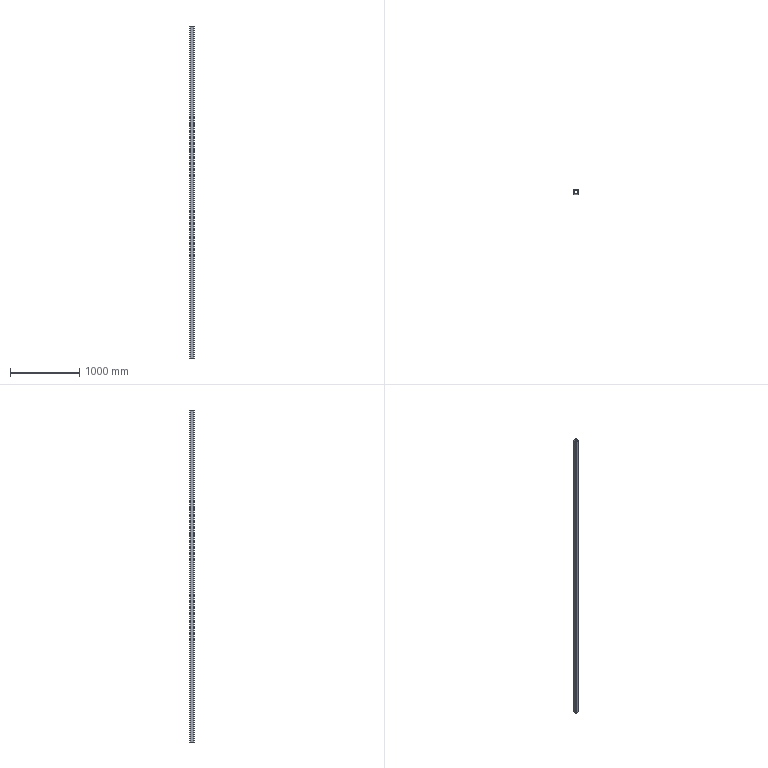Part | SolidWorks | features Extrusion 1 | 1 solid | 18 faces | box 64 x 64 x 4800 mm | volume 4410223 mm3 | plane 10 | cylinder 8 | commonest cylinder face diameters 8 x4 16 x4
STEP:
#1=CARTESIAN_POINT('',(-24.,32.,2400.));
#2=VERTEX_POINT('',#1);
#3=CARTESIAN_POINT('',(-32.,24.,2400.));
#4=VERTEX_POINT('',#3);
#5=CARTESIAN_POINT('',(-24.,24.,2400.));
#6=DIRECTION('',(0.,0.,1.));
#7=DIRECTION('',(1.,0.,0.));
#8=AXIS2_PLACEMENT_3D('',#5,#6,#7);
#9=CIRCLE('',#8,8.);
#10=EDGE_CURVE('',#2,#4,#9,.T.);
#11=ORIENTED_EDGE('',*,*,#10,.T.);
#12=CARTESIAN_POINT('',(-32.,-24.,2400.));
#13=VERTEX_POINT('',#12);
#14=CARTESIAN_POINT('',(-32.,24.,2400.));
#15=DIRECTION('',(0.,-1.,0.));
#16=VECTOR('',#15,1000.);
#17=LINE('',#14,#16);
#18=EDGE_CURVE('',#4,#13,#17,.T.);
#19=ORIENTED_EDGE('',*,*,#18,.T.);
#20=CARTESIAN_POINT('',(-24.,-32.,2400.));
#21=VERTEX_POINT('',#20);
#22=CARTESIAN_POINT('',(-24.,-24.,2400.));
#23=DIRECTION('',(0.,0.,1.));
#24=DIRECTION('',(-1.,0.,0.));
#25=AXIS2_PLACEMENT_3D('',#22,#23,#24);
#26=CIRCLE('',#25,8.);
#27=EDGE_CURVE('',#13,#21,#26,.T.);
#28=ORIENTED_EDGE('',*,*,#27,.T.);
#29=CARTESIAN_POINT('',(24.,-32.,2400.));
#30=VERTEX_POINT('',#29);
#31=CARTESIAN_POINT('',(24.,-32.,2400.));
#32=DIRECTION('',(1.,0.,0.));
#33=VECTOR('',#32,1000.);
#34=LINE('',#31,#33);
#35=EDGE_CURVE('',#21,#30,#34,.T.);
#36=ORIENTED_EDGE('',*,*,#35,.T.);
#37=CARTESIAN_POINT('',(32.,-24.,2400.));
#38=VERTEX_POINT('',#37);
#39=CARTESIAN_POINT('',(24.,-24.,2400.));
#40=DIRECTION('',(0.,0.,1.));
#41=DIRECTION('',(1.,0.,0.));
#42=AXIS2_PLACEMENT_3D('',#39,#40,#41);
#43=CIRCLE('',#42,8.);
#44=EDGE_CURVE('',#30,#38,#43,.T.);
#45=ORIENTED_EDGE('',*,*,#44,.T.);
#46=CARTESIAN_POINT('',(32.,24.,2400.));
#47=VERTEX_POINT('',#46);
#48=CARTESIAN_POINT('',(32.,-24.,2400.));
#49=DIRECTION('',(0.,1.,0.));
#50=VECTOR('',#49,1000.);
#51=LINE('',#48,#50);
#52=EDGE_CURVE('',#38,#47,#51,.T.);
#53=ORIENTED_EDGE('',*,*,#52,.T.);
#54=CARTESIAN_POINT('',(24.,32.,2400.));
#55=VERTEX_POINT('',#54);
#56=CARTESIAN_POINT('',(24.,24.,2400.));
#57=DIRECTION('',(0.,0.,1.));
#58=DIRECTION('',(-1.,0.,0.));
#59=AXIS2_PLACEMENT_3D('',#56,#57,#58);
#60=CIRCLE('',#59,8.);
#61=EDGE_CURVE('',#47,#55,#60,.T.);
#62=ORIENTED_EDGE('',*,*,#61,.T.);
#63=CARTESIAN_POINT('',(0.,32.,2400.));
#64=DIRECTION('',(-1.,0.,0.));
#65=VECTOR('',#64,1000.);
#66=LINE('',#63,#65);
#67=EDGE_CURVE('',#55,#2,#66,.T.);
#68=ORIENTED_EDGE('',*,*,#67,.T.);
#69=EDGE_LOOP('',(#11,#19,#28,#36,#45,#53,#62,#68));
#70=FACE_OUTER_BOUND('',#69,.T.);
#71=CARTESIAN_POINT('',(-28.,24.,2400.));
#72=VERTEX_POINT('',#71);
#73=CARTESIAN_POINT('',(-28.,-24.,2400.));
#74=VERTEX_POINT('',#73);
#75=CARTESIAN_POINT('',(-28.,24.,2400.));
#76=DIRECTION('',(0.,-1.,0.));
#77=VECTOR('',#76,1000.);
#78=LINE('',#75,#77);
#79=EDGE_CURVE('',#72,#74,#78,.T.);
#80=ORIENTED_EDGE('',*,*,#79,.F.);
#81=CARTESIAN_POINT('',(-24.,28.,2400.));
#82=VERTEX_POINT('',#81);
#83=CARTESIAN_POINT('',(-24.,24.,2400.));
#84=DIRECTION('',(0.,0.,1.));
#85=DIRECTION('',(1.,0.,0.));
#86=AXIS2_PLACEMENT_3D('',#83,#84,#85);
#87=CIRCLE('',#86,4.);
#88=EDGE_CURVE('',#82,#72,#87,.T.);
#89=ORIENTED_EDGE('',*,*,#88,.F.);
#90=CARTESIAN_POINT('',(24.,28.,2400.));
#91=VERTEX_POINT('',#90);
#92=CARTESIAN_POINT('',(0.,28.,2400.));
#93=DIRECTION('',(-1.,0.,0.));
#94=VECTOR('',#93,1000.);
#95=LINE('',#92,#94);
#96=EDGE_CURVE('',#91,#82,#95,.T.);
#97=ORIENTED_EDGE('',*,*,#96,.F.);
#98=CARTESIAN_POINT('',(28.,24.,2400.));
#99=VERTEX_POINT('',#98);
#100=CARTESIAN_POINT('',(24.,24.,2400.));
#101=DIRECTION('',(0.,0.,1.));
#102=DIRECTION('',(-1.,0.,0.));
#103=AXIS2_PLACEMENT_3D('',#100,#101,#102);
#104=CIRCLE('',#103,4.);
#105=EDGE_CURVE('',#99,#91,#104,.T.);
#106=ORIENTED_EDGE('',*,*,#105,.F.);
#107=CARTESIAN_POINT('',(28.,-24.,2400.));
#108=VERTEX_POINT('',#107);
#109=CARTESIAN_POINT('',(28.,-24.,2400.));
#110=DIRECTION('',(0.,1.,0.));
#111=VECTOR('',#110,1000.);
#112=LINE('',#109,#111);
#113=EDGE_CURVE('',#108,#99,#112,.T.);
#114=ORIENTED_EDGE('',*,*,#113,.F.);
#115=CARTESIAN_POINT('',(24.,-28.,2400.));
#116=VERTEX_POINT('',#115);
#117=CARTESIAN_POINT('',(24.,-24.,2400.));
#118=DIRECTION('',(0.,0.,1.));
#119=DIRECTION('',(1.,0.,0.));
#120=AXIS2_PLACEMENT_3D('',#117,#118,#119);
#121=CIRCLE('',#120,4.);
#122=EDGE_CURVE('',#116,#108,#121,.T.);
#123=ORIENTED_EDGE('',*,*,#122,.F.);
#124=CARTESIAN_POINT('',(-24.,-28.,2400.));
#125=VERTEX_POINT('',#124);
#126=CARTESIAN_POINT('',(24.,-28.,2400.));
#127=DIRECTION('',(1.,0.,0.));
#128=VECTOR('',#127,1000.);
#129=LINE('',#126,#128);
#130=EDGE_CURVE('',#125,#116,#129,.T.);
#131=ORIENTED_EDGE('',*,*,#130,.F.);
#132=CARTESIAN_POINT('',(-24.,-24.,2400.));
#133=DIRECTION('',(0.,0.,1.));
#134=DIRECTION('',(-1.,0.,0.));
#135=AXIS2_PLACEMENT_3D('',#132,#133,#134);
#136=CIRCLE('',#135,4.);
#137=EDGE_CURVE('',#74,#125,#136,.T.);
#138=ORIENTED_EDGE('',*,*,#137,.F.);
#139=EDGE_LOOP('',(#80,#89,#97,#106,#114,#123,#131,#138));
#140=FACE_BOUND('',#139,.T.);
#141=CARTESIAN_POINT('',(-24.,24.,2400.));
#142=DIRECTION('',(0.,0.,1.));
#143=DIRECTION('',(1.,0.,0.));
#144=AXIS2_PLACEMENT_3D('',#141,#142,#143);
#145=PLANE('',#144);
#146=ADVANCED_FACE('',(#70,#140),#145,.T.);
#147=CARTESIAN_POINT('',(-24.,32.,-2400.));
#148=VERTEX_POINT('',#147);
#149=CARTESIAN_POINT('',(-32.,24.,-2400.));
#150=VERTEX_POINT('',#149);
#151=CARTESIAN_POINT('',(-24.,24.,-2400.));
#152=DIRECTION('',(0.,0.,1.));
#153=DIRECTION('',(1.,0.,0.));
#154=AXIS2_PLACEMENT_3D('',#151,#152,#153);
#155=CIRCLE('',#154,8.);
#156=EDGE_CURVE('',#148,#150,#155,.T.);
#157=ORIENTED_EDGE('',*,*,#156,.F.);
#158=CARTESIAN_POINT('',(24.,32.,-2400.));
#159=VERTEX_POINT('',#158);
#160=CARTESIAN_POINT('',(0.,32.,-2400.));
#161=DIRECTION('',(-1.,0.,0.));
#162=VECTOR('',#161,1000.);
#163=LINE('',#160,#162);
#164=EDGE_CURVE('',#159,#148,#163,.T.);
#165=ORIENTED_EDGE('',*,*,#164,.F.);
#166=CARTESIAN_POINT('',(32.,24.,-2400.));
#167=VERTEX_POINT('',#166);
#168=CARTESIAN_POINT('',(24.,24.,-2400.));
#169=DIRECTION('',(0.,0.,1.));
#170=DIRECTION('',(-1.,0.,0.));
#171=AXIS2_PLACEMENT_3D('',#168,#169,#170);
#172=CIRCLE('',#171,8.);
#173=EDGE_CURVE('',#167,#159,#172,.T.);
#174=ORIENTED_EDGE('',*,*,#173,.F.);
#175=CARTESIAN_POINT('',(32.,-24.,-2400.));
#176=VERTEX_POINT('',#175);
#177=CARTESIAN_POINT('',(32.,24.,-2400.));
#178=DIRECTION('',(0.,1.,0.));
#179=VECTOR('',#178,1000.);
#180=LINE('',#177,#179);
#181=EDGE_CURVE('',#176,#167,#180,.T.);
#182=ORIENTED_EDGE('',*,*,#181,.F.);
#183=CARTESIAN_POINT('',(24.,-32.,-2400.));
#184=VERTEX_POINT('',#183);
#185=CARTESIAN_POINT('',(24.,-24.,-2400.));
#186=DIRECTION('',(0.,0.,1.));
#187=DIRECTION('',(1.,0.,0.));
#188=AXIS2_PLACEMENT_3D('',#185,#186,#187);
#189=CIRCLE('',#188,8.);
#190=EDGE_CURVE('',#184,#176,#189,.T.);
#191=ORIENTED_EDGE('',*,*,#190,.F.);
#192=CARTESIAN_POINT('',(-24.,-32.,-2400.));
#193=VERTEX_POINT('',#192);
#194=CARTESIAN_POINT('',(24.,-32.,-2400.));
#195=DIRECTION('',(1.,0.,0.));
#196=VECTOR('',#195,1000.);
#197=LINE('',#194,#196);
#198=EDGE_CURVE('',#193,#184,#197,.T.);
#199=ORIENTED_EDGE('',*,*,#198,.F.);
#200=CARTESIAN_POINT('',(-32.,-24.,-2400.));
#201=VERTEX_POINT('',#200);
#202=CARTESIAN_POINT('',(-24.,-24.,-2400.));
#203=DIRECTION('',(0.,0.,1.));
#204=DIRECTION('',(-1.,0.,0.));
#205=AXIS2_PLACEMENT_3D('',#202,#203,#204);
#206=CIRCLE('',#205,8.);
#207=EDGE_CURVE('',#201,#193,#206,.T.);
#208=ORIENTED_EDGE('',*,*,#207,.F.);
#209=CARTESIAN_POINT('',(-32.,-24.,-2400.));
#210=DIRECTION('',(0.,-1.,0.));
#211=VECTOR('',#210,1000.);
#212=LINE('',#209,#211);
#213=EDGE_CURVE('',#150,#201,#212,.T.);
#214=ORIENTED_EDGE('',*,*,#213,.F.);
#215=EDGE_LOOP('',(#157,#165,#174,#182,#191,#199,#208,#214));
#216=FACE_OUTER_BOUND('',#215,.T.);
#217=CARTESIAN_POINT('',(-24.,28.,-2400.));
#218=VERTEX_POINT('',#217);
#219=CARTESIAN_POINT('',(-28.,24.,-2400.));
#220=VERTEX_POINT('',#219);
#221=CARTESIAN_POINT('',(-24.,24.,-2400.));
#222=DIRECTION('',(0.,0.,1.));
#223=DIRECTION('',(1.,0.,0.));
#224=AXIS2_PLACEMENT_3D('',#221,#222,#223);
#225=CIRCLE('',#224,4.);
#226=EDGE_CURVE('',#218,#220,#225,.T.);
#227=ORIENTED_EDGE('',*,*,#226,.T.);
#228=CARTESIAN_POINT('',(-28.,-24.,-2400.));
#229=VERTEX_POINT('',#228);
#230=CARTESIAN_POINT('',(-28.,-24.,-2400.));
#231=DIRECTION('',(0.,-1.,0.));
#232=VECTOR('',#231,1000.);
#233=LINE('',#230,#232);
#234=EDGE_CURVE('',#220,#229,#233,.T.);
#235=ORIENTED_EDGE('',*,*,#234,.T.);
#236=CARTESIAN_POINT('',(-24.,-28.,-2400.));
#237=VERTEX_POINT('',#236);
#238=CARTESIAN_POINT('',(-24.,-24.,-2400.));
#239=DIRECTION('',(0.,0.,1.));
#240=DIRECTION('',(-1.,0.,0.));
#241=AXIS2_PLACEMENT_3D('',#238,#239,#240);
#242=CIRCLE('',#241,4.);
#243=EDGE_CURVE('',#229,#237,#242,.T.);
#244=ORIENTED_EDGE('',*,*,#243,.T.);
#245=CARTESIAN_POINT('',(24.,-28.,-2400.));
#246=VERTEX_POINT('',#245);
#247=CARTESIAN_POINT('',(24.,-28.,-2400.));
#248=DIRECTION('',(1.,0.,0.));
#249=VECTOR('',#248,1000.);
#250=LINE('',#247,#249);
#251=EDGE_CURVE('',#237,#246,#250,.T.);
#252=ORIENTED_EDGE('',*,*,#251,.T.);
#253=CARTESIAN_POINT('',(28.,-24.,-2400.));
#254=VERTEX_POINT('',#253);
#255=CARTESIAN_POINT('',(24.,-24.,-2400.));
#256=DIRECTION('',(0.,0.,1.));
#257=DIRECTION('',(1.,0.,0.));
#258=AXIS2_PLACEMENT_3D('',#255,#256,#257);
#259=CIRCLE('',#258,4.);
#260=EDGE_CURVE('',#246,#254,#259,.T.);
#261=ORIENTED_EDGE('',*,*,#260,.T.);
#262=CARTESIAN_POINT('',(28.,24.,-2400.));
#263=VERTEX_POINT('',#262);
#264=CARTESIAN_POINT('',(28.,24.,-2400.));
#265=DIRECTION('',(0.,1.,0.));
#266=VECTOR('',#265,1000.);
#267=LINE('',#264,#266);
#268=EDGE_CURVE('',#254,#263,#267,.T.);
#269=ORIENTED_EDGE('',*,*,#268,.T.);
#270=CARTESIAN_POINT('',(24.,28.,-2400.));
#271=VERTEX_POINT('',#270);
#272=CARTESIAN_POINT('',(24.,24.,-2400.));
#273=DIRECTION('',(0.,0.,1.));
#274=DIRECTION('',(-1.,0.,0.));
#275=AXIS2_PLACEMENT_3D('',#272,#273,#274);
#276=CIRCLE('',#275,4.);
#277=EDGE_CURVE('',#263,#271,#276,.T.);
#278=ORIENTED_EDGE('',*,*,#277,.T.);
#279=CARTESIAN_POINT('',(0.,28.,-2400.));
#280=DIRECTION('',(-1.,0.,0.));
#281=VECTOR('',#280,1000.);
#282=LINE('',#279,#281);
#283=EDGE_CURVE('',#271,#218,#282,.T.);
#284=ORIENTED_EDGE('',*,*,#283,.T.);
#285=EDGE_LOOP('',(#227,#235,#244,#252,#261,#269,#278,#284));
#286=FACE_BOUND('',#285,.T.);
#287=CARTESIAN_POINT('',(-24.,24.,-2400.));
#288=DIRECTION('',(0.,0.,1.));
#289=DIRECTION('',(1.,0.,0.));
#290=AXIS2_PLACEMENT_3D('',#287,#288,#289);
#291=PLANE('',#290);
#292=ADVANCED_FACE('',(#216,#286),#291,.F.);
#293=ORIENTED_EDGE('',*,*,#156,.T.);
#294=CARTESIAN_POINT('',(-32.,24.,2400.));
#295=DIRECTION('',(0.,0.,-1.));
#296=VECTOR('',#295,1000.);
#297=LINE('',#294,#296);
#298=EDGE_CURVE('',#4,#150,#297,.T.);
#299=ORIENTED_EDGE('',*,*,#298,.F.);
#300=ORIENTED_EDGE('',*,*,#10,.F.);
#301=CARTESIAN_POINT('',(-24.,32.,2400.));
#302=DIRECTION('',(0.,0.,-1.));
#303=VECTOR('',#302,1000.);
#304=LINE('',#301,#303);
#305=EDGE_CURVE('',#2,#148,#304,.T.);
#306=ORIENTED_EDGE('',*,*,#305,.T.);
#307=EDGE_LOOP('',(#293,#299,#300,#306));
#308=FACE_OUTER_BOUND('',#307,.T.);
#309=CARTESIAN_POINT('',(-24.,24.,2400.));
#310=DIRECTION('',(0.,0.,-1.));
#311=DIRECTION('',(-1.,0.,0.));
#312=AXIS2_PLACEMENT_3D('',#309,#310,#311);
#313=CYLINDRICAL_SURFACE('',#312,8.);
#314=ADVANCED_FACE('',(#308),#313,.T.);
#315=ORIENTED_EDGE('',*,*,#213,.T.);
#316=CARTESIAN_POINT('',(-32.,-24.,2400.));
#317=DIRECTION('',(0.,0.,-1.));
#318=VECTOR('',#317,1000.);
#319=LINE('',#316,#318);
#320=EDGE_CURVE('',#13,#201,#319,.T.);
#321=ORIENTED_EDGE('',*,*,#320,.F.);
#322=ORIENTED_EDGE('',*,*,#18,.F.);
#323=ORIENTED_EDGE('',*,*,#298,.T.);
#324=EDGE_LOOP('',(#315,#321,#322,#323));
#325=FACE_OUTER_BOUND('',#324,.T.);
#326=CARTESIAN_POINT('',(-32.,-24.,2400.));
#327=DIRECTION('',(1.,0.,0.));
#328=DIRECTION('',(0.,0.,-1.));
#329=AXIS2_PLACEMENT_3D('',#326,#327,#328);
#330=PLANE('',#329);
#331=ADVANCED_FACE('',(#325),#330,.F.);
#332=ORIENTED_EDGE('',*,*,#207,.T.);
#333=CARTESIAN_POINT('',(-24.,-32.,2400.));
#334=DIRECTION('',(0.,0.,-1.));
#335=VECTOR('',#334,1000.);
#336=LINE('',#333,#335);
#337=EDGE_CURVE('',#21,#193,#336,.T.);
#338=ORIENTED_EDGE('',*,*,#337,.F.);
#339=ORIENTED_EDGE('',*,*,#27,.F.);
#340=ORIENTED_EDGE('',*,*,#320,.T.);
#341=EDGE_LOOP('',(#332,#338,#339,#340));
#342=FACE_OUTER_BOUND('',#341,.T.);
#343=CARTESIAN_POINT('',(-24.,-24.,2400.));
#344=DIRECTION('',(0.,0.,-1.));
#345=DIRECTION('',(-1.,0.,0.));
#346=AXIS2_PLACEMENT_3D('',#343,#344,#345);
#347=CYLINDRICAL_SURFACE('',#346,8.);
#348=ADVANCED_FACE('',(#342),#347,.T.);
#349=ORIENTED_EDGE('',*,*,#198,.T.);
#350=CARTESIAN_POINT('',(24.,-32.,2400.));
#351=DIRECTION('',(0.,0.,-1.));
#352=VECTOR('',#351,1000.);
#353=LINE('',#350,#352);
#354=EDGE_CURVE('',#30,#184,#353,.T.);
#355=ORIENTED_EDGE('',*,*,#354,.F.);
#356=ORIENTED_EDGE('',*,*,#35,.F.);
#357=ORIENTED_EDGE('',*,*,#337,.T.);
#358=EDGE_LOOP('',(#349,#355,#356,#357));
#359=FACE_OUTER_BOUND('',#358,.T.);
#360=CARTESIAN_POINT('',(24.,-32.,2400.));
#361=DIRECTION('',(0.,1.,0.));
#362=DIRECTION('',(-1.,0.,0.));
#363=AXIS2_PLACEMENT_3D('',#360,#361,#362);
#364=PLANE('',#363);
#365=ADVANCED_FACE('',(#359),#364,.F.);
#366=ORIENTED_EDGE('',*,*,#190,.T.);
#367=CARTESIAN_POINT('',(32.,-24.,2400.));
#368=DIRECTION('',(0.,0.,-1.));
#369=VECTOR('',#368,1000.);
#370=LINE('',#367,#369);
#371=EDGE_CURVE('',#38,#176,#370,.T.);
#372=ORIENTED_EDGE('',*,*,#371,.F.);
#373=ORIENTED_EDGE('',*,*,#44,.F.);
#374=ORIENTED_EDGE('',*,*,#354,.T.);
#375=EDGE_LOOP('',(#366,#372,#373,#374));
#376=FACE_OUTER_BOUND('',#375,.T.);
#377=CARTESIAN_POINT('',(24.,-24.,2400.));
#378=DIRECTION('',(0.,0.,-1.));
#379=DIRECTION('',(-1.,0.,0.));
#380=AXIS2_PLACEMENT_3D('',#377,#378,#379);
#381=CYLINDRICAL_SURFACE('',#380,8.);
#382=ADVANCED_FACE('',(#376),#381,.T.);
#383=ORIENTED_EDGE('',*,*,#181,.T.);
#384=CARTESIAN_POINT('',(32.,24.,2400.));
#385=DIRECTION('',(0.,0.,-1.));
#386=VECTOR('',#385,1000.);
#387=LINE('',#384,#386);
#388=EDGE_CURVE('',#47,#167,#387,.T.);
#389=ORIENTED_EDGE('',*,*,#388,.F.);
#390=ORIENTED_EDGE('',*,*,#52,.F.);
#391=ORIENTED_EDGE('',*,*,#371,.T.);
#392=EDGE_LOOP('',(#383,#389,#390,#391));
#393=FACE_OUTER_BOUND('',#392,.T.);
#394=CARTESIAN_POINT('',(32.,24.,2400.));
#395=DIRECTION('',(-1.,0.,0.));
#396=DIRECTION('',(0.,0.,1.));
#397=AXIS2_PLACEMENT_3D('',#394,#395,#396);
#398=PLANE('',#397);
#399=ADVANCED_FACE('',(#393),#398,.F.);
#400=ORIENTED_EDGE('',*,*,#173,.T.);
#401=CARTESIAN_POINT('',(24.,32.,2400.));
#402=DIRECTION('',(0.,0.,-1.));
#403=VECTOR('',#402,1000.);
#404=LINE('',#401,#403);
#405=EDGE_CURVE('',#55,#159,#404,.T.);
#406=ORIENTED_EDGE('',*,*,#405,.F.);
#407=ORIENTED_EDGE('',*,*,#61,.F.);
#408=ORIENTED_EDGE('',*,*,#388,.T.);
#409=EDGE_LOOP('',(#400,#406,#407,#408));
#410=FACE_OUTER_BOUND('',#409,.T.);
#411=CARTESIAN_POINT('',(24.,24.,2400.));
#412=DIRECTION('',(0.,0.,-1.));
#413=DIRECTION('',(-1.,0.,0.));
#414=AXIS2_PLACEMENT_3D('',#411,#412,#413);
#415=CYLINDRICAL_SURFACE('',#414,8.);
#416=ADVANCED_FACE('',(#410),#415,.T.);
#417=ORIENTED_EDGE('',*,*,#164,.T.);
#418=ORIENTED_EDGE('',*,*,#305,.F.);
#419=ORIENTED_EDGE('',*,*,#67,.F.);
#420=ORIENTED_EDGE('',*,*,#405,.T.);
#421=EDGE_LOOP('',(#417,#418,#419,#420));
#422=FACE_OUTER_BOUND('',#421,.T.);
#423=CARTESIAN_POINT('',(0.,32.,2400.));
#424=DIRECTION('',(0.,-1.,0.));
#425=DIRECTION('',(0.,0.,-1.));
#426=AXIS2_PLACEMENT_3D('',#423,#424,#425);
#427=PLANE('',#426);
#428=ADVANCED_FACE('',(#422),#427,.F.);
#429=ORIENTED_EDGE('',*,*,#226,.F.);
#430=CARTESIAN_POINT('',(-24.,28.,2400.));
#431=DIRECTION('',(0.,0.,-1.));
#432=VECTOR('',#431,1000.);
#433=LINE('',#430,#432);
#434=EDGE_CURVE('',#82,#218,#433,.T.);
#435=ORIENTED_EDGE('',*,*,#434,.F.);
#436=ORIENTED_EDGE('',*,*,#88,.T.);
#437=CARTESIAN_POINT('',(-28.,24.,2400.));
#438=DIRECTION('',(0.,0.,-1.));
#439=VECTOR('',#438,1000.);
#440=LINE('',#437,#439);
#441=EDGE_CURVE('',#72,#220,#440,.T.);
#442=ORIENTED_EDGE('',*,*,#441,.T.);
#443=EDGE_LOOP('',(#429,#435,#436,#442));
#444=FACE_OUTER_BOUND('',#443,.T.);
#445=CARTESIAN_POINT('',(-24.,24.,2400.));
#446=DIRECTION('',(0.,0.,-1.));
#447=DIRECTION('',(-1.,0.,0.));
#448=AXIS2_PLACEMENT_3D('',#445,#446,#447);
#449=CYLINDRICAL_SURFACE('',#448,4.);
#450=ADVANCED_FACE('',(#444),#449,.F.);
#451=ORIENTED_EDGE('',*,*,#234,.F.);
#452=ORIENTED_EDGE('',*,*,#441,.F.);
#453=ORIENTED_EDGE('',*,*,#79,.T.);
#454=CARTESIAN_POINT('',(-28.,-24.,2400.));
#455=DIRECTION('',(0.,0.,-1.));
#456=VECTOR('',#455,1000.);
#457=LINE('',#454,#456);
#458=EDGE_CURVE('',#74,#229,#457,.T.);
#459=ORIENTED_EDGE('',*,*,#458,.T.);
#460=EDGE_LOOP('',(#451,#452,#453,#459));
#461=FACE_OUTER_BOUND('',#460,.T.);
#462=CARTESIAN_POINT('',(-28.,-24.,2400.));
#463=DIRECTION('',(1.,0.,0.));
#464=DIRECTION('',(0.,1.,0.));
#465=AXIS2_PLACEMENT_3D('',#462,#463,#464);
#466=PLANE('',#465);
#467=ADVANCED_FACE('',(#461),#466,.T.);
#468=ORIENTED_EDGE('',*,*,#243,.F.);
#469=ORIENTED_EDGE('',*,*,#458,.F.);
#470=ORIENTED_EDGE('',*,*,#137,.T.);
#471=CARTESIAN_POINT('',(-24.,-28.,2400.));
#472=DIRECTION('',(0.,0.,-1.));
#473=VECTOR('',#472,1000.);
#474=LINE('',#471,#473);
#475=EDGE_CURVE('',#125,#237,#474,.T.);
#476=ORIENTED_EDGE('',*,*,#475,.T.);
#477=EDGE_LOOP('',(#468,#469,#470,#476));
#478=FACE_OUTER_BOUND('',#477,.T.);
#479=CARTESIAN_POINT('',(-24.,-24.,2400.));
#480=DIRECTION('',(0.,0.,-1.));
#481=DIRECTION('',(-1.,0.,0.));
#482=AXIS2_PLACEMENT_3D('',#479,#480,#481);
#483=CYLINDRICAL_SURFACE('',#482,4.);
#484=ADVANCED_FACE('',(#478),#483,.F.);
#485=ORIENTED_EDGE('',*,*,#251,.F.);
#486=ORIENTED_EDGE('',*,*,#475,.F.);
#487=ORIENTED_EDGE('',*,*,#130,.T.);
#488=CARTESIAN_POINT('',(24.,-28.,2400.));
#489=DIRECTION('',(0.,0.,-1.));
#490=VECTOR('',#489,1000.);
#491=LINE('',#488,#490);
#492=EDGE_CURVE('',#116,#246,#491,.T.);
#493=ORIENTED_EDGE('',*,*,#492,.T.);
#494=EDGE_LOOP('',(#485,#486,#487,#493));
#495=FACE_OUTER_BOUND('',#494,.T.);
#496=CARTESIAN_POINT('',(24.,-28.,2400.));
#497=DIRECTION('',(0.,1.,0.));
#498=DIRECTION('',(-1.,0.,0.));
#499=AXIS2_PLACEMENT_3D('',#496,#497,#498);
#500=PLANE('',#499);
#501=ADVANCED_FACE('',(#495),#500,.T.);
#502=ORIENTED_EDGE('',*,*,#260,.F.);
#503=ORIENTED_EDGE('',*,*,#492,.F.);
#504=ORIENTED_EDGE('',*,*,#122,.T.);
#505=CARTESIAN_POINT('',(28.,-24.,2400.));
#506=DIRECTION('',(0.,0.,-1.));
#507=VECTOR('',#506,1000.);
#508=LINE('',#505,#507);
#509=EDGE_CURVE('',#108,#254,#508,.T.);
#510=ORIENTED_EDGE('',*,*,#509,.T.);
#511=EDGE_LOOP('',(#502,#503,#504,#510));
#512=FACE_OUTER_BOUND('',#511,.T.);
#513=CARTESIAN_POINT('',(24.,-24.,2400.));
#514=DIRECTION('',(0.,0.,-1.));
#515=DIRECTION('',(-1.,0.,0.));
#516=AXIS2_PLACEMENT_3D('',#513,#514,#515);
#517=CYLINDRICAL_SURFACE('',#516,4.);
#518=ADVANCED_FACE('',(#512),#517,.F.);
#519=ORIENTED_EDGE('',*,*,#268,.F.);
#520=ORIENTED_EDGE('',*,*,#509,.F.);
#521=ORIENTED_EDGE('',*,*,#113,.T.);
#522=CARTESIAN_POINT('',(28.,24.,2400.));
#523=DIRECTION('',(0.,0.,-1.));
#524=VECTOR('',#523,1000.);
#525=LINE('',#522,#524);
#526=EDGE_CURVE('',#99,#263,#525,.T.);
#527=ORIENTED_EDGE('',*,*,#526,.T.);
#528=EDGE_LOOP('',(#519,#520,#521,#527));
#529=FACE_OUTER_BOUND('',#528,.T.);
#530=CARTESIAN_POINT('',(28.,24.,2400.));
#531=DIRECTION('',(-1.,0.,0.));
#532=DIRECTION('',(0.,-1.,0.));
#533=AXIS2_PLACEMENT_3D('',#530,#531,#532);
#534=PLANE('',#533);
#535=ADVANCED_FACE('',(#529),#534,.T.);
#536=ORIENTED_EDGE('',*,*,#277,.F.);
#537=ORIENTED_EDGE('',*,*,#526,.F.);
#538=ORIENTED_EDGE('',*,*,#105,.T.);
#539=CARTESIAN_POINT('',(24.,28.,2400.));
#540=DIRECTION('',(0.,0.,-1.));
#541=VECTOR('',#540,1000.);
#542=LINE('',#539,#541);
#543=EDGE_CURVE('',#91,#271,#542,.T.);
#544=ORIENTED_EDGE('',*,*,#543,.T.);
#545=EDGE_LOOP('',(#536,#537,#538,#544));
#546=FACE_OUTER_BOUND('',#545,.T.);
#547=CARTESIAN_POINT('',(24.,24.,2400.));
#548=DIRECTION('',(0.,0.,-1.));
#549=DIRECTION('',(-1.,0.,0.));
#550=AXIS2_PLACEMENT_3D('',#547,#548,#549);
#551=CYLINDRICAL_SURFACE('',#550,4.);
#552=ADVANCED_FACE('',(#546),#551,.F.);
#553=ORIENTED_EDGE('',*,*,#283,.F.);
#554=ORIENTED_EDGE('',*,*,#543,.F.);
#555=ORIENTED_EDGE('',*,*,#96,.T.);
#556=ORIENTED_EDGE('',*,*,#434,.T.);
#557=EDGE_LOOP('',(#553,#554,#555,#556));
#558=FACE_OUTER_BOUND('',#557,.T.);
#559=CARTESIAN_POINT('',(0.,28.,2400.));
#560=DIRECTION('',(0.,-1.,0.));
#561=DIRECTION('',(0.,0.,-1.));
#562=AXIS2_PLACEMENT_3D('',#559,#560,#561);
#563=PLANE('',#562);
#564=ADVANCED_FACE('',(#558),#563,.T.);
#565=CLOSED_SHELL('',(#146,#292,#314,#331,#348,#365,#382,#399,#416,#428,#450,#467,#484,#501,#518,#535,#552,#564));
#566=MANIFOLD_SOLID_BREP('',#565);
#567=CARTESIAN_POINT('',(0.,0.,0.));
#568=DIRECTION('',(0.,0.,1.));
#569=DIRECTION('',(1.,0.,0.));
#570=AXIS2_PLACEMENT_3D('',#567,#568,#569);
#571=(LENGTH_UNIT()NAMED_UNIT(*)SI_UNIT(.MILLI.,.METRE.));
#572=UNCERTAINTY_MEASURE_WITH_UNIT(LENGTH_MEASURE(0.00001),#571,'','');
#573=(NAMED_UNIT(*)PLANE_ANGLE_UNIT()SI_UNIT($,.RADIAN.));
#574=(NAMED_UNIT(*)SI_UNIT($,.STERADIAN.)SOLID_ANGLE_UNIT());
#575=(GEOMETRIC_REPRESENTATION_CONTEXT(3)GLOBAL_UNCERTAINTY_ASSIGNED_CONTEXT((#572))GLOBAL_UNIT_ASSIGNED_CONTEXT((#571,#573,#574))REPRESENTATION_CONTEXT('',''));
#576=ADVANCED_BREP_SHAPE_REPRESENTATION('',(#566,#570),#575);